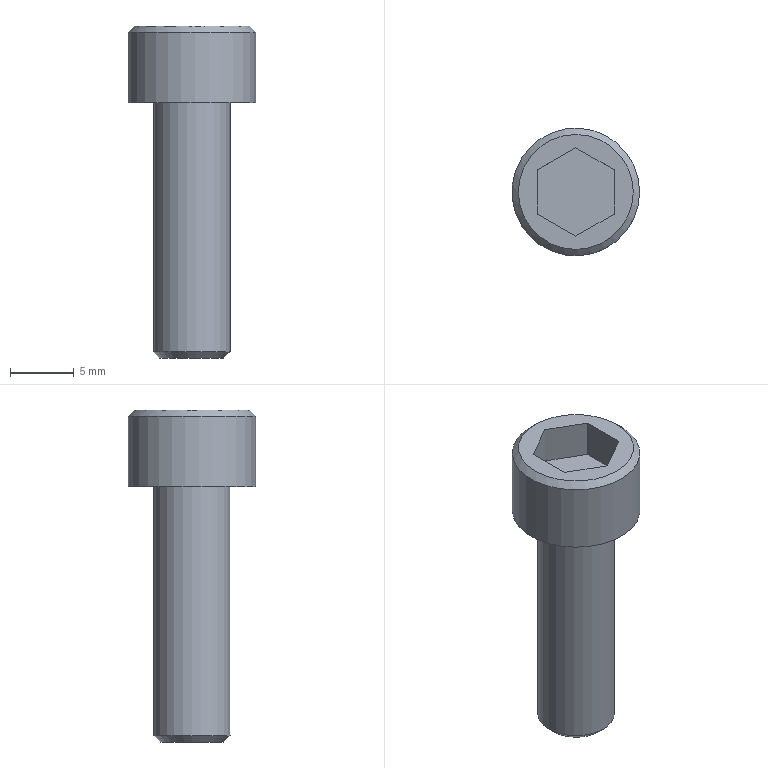Part | NX | features solid 2 | 1 solid | 14 faces | box 10 x 10 x 26 mm | volume 937.173 mm3 | plane 10 | cylinder 2 | cone 2 | commonest cylinder face diameters 6 x1 10 x1
STEP:
#1=CARTESIAN_POINT('',(47.,0.,109.5));
#2=VERTEX_POINT('',#1);
#3=CARTESIAN_POINT('',(42.5,0.,109.5));
#4=DIRECTION('',(0.,0.,1.));
#5=DIRECTION('',(1.,0.,0.));
#6=AXIS2_PLACEMENT_3D('',#3,#4,#5);
#7=CIRCLE('',#6,4.5);
#8=EDGE_CURVE('',#2,#2,#7,.T.);
#9=ORIENTED_EDGE('',*,*,#8,.T.);
#10=EDGE_LOOP('',(#9));
#11=FACE_BOUND('',#10,.T.);
#12=CARTESIAN_POINT('',(45.5,-1.732,109.5));
#13=VERTEX_POINT('',#12);
#14=CARTESIAN_POINT('',(42.5,-3.464,109.5));
#15=VERTEX_POINT('',#14);
#16=CARTESIAN_POINT('',(45.5,-1.732,109.5));
#17=DIRECTION('',(-0.866,-0.5,0.));
#18=VECTOR('',#17,1000.);
#19=LINE('',#16,#18);
#20=EDGE_CURVE('',#13,#15,#19,.T.);
#21=ORIENTED_EDGE('',*,*,#20,.T.);
#22=CARTESIAN_POINT('',(39.5,-1.732,109.5));
#23=VERTEX_POINT('',#22);
#24=CARTESIAN_POINT('',(42.5,-3.464,109.5));
#25=DIRECTION('',(-0.866,0.5,0.));
#26=VECTOR('',#25,1000.);
#27=LINE('',#24,#26);
#28=EDGE_CURVE('',#15,#23,#27,.T.);
#29=ORIENTED_EDGE('',*,*,#28,.T.);
#30=CARTESIAN_POINT('',(39.5,1.732,109.5));
#31=VERTEX_POINT('',#30);
#32=CARTESIAN_POINT('',(39.5,-1.732,109.5));
#33=DIRECTION('',(0.,1.,0.));
#34=VECTOR('',#33,1000.);
#35=LINE('',#32,#34);
#36=EDGE_CURVE('',#23,#31,#35,.T.);
#37=ORIENTED_EDGE('',*,*,#36,.T.);
#38=CARTESIAN_POINT('',(42.5,3.464,109.5));
#39=VERTEX_POINT('',#38);
#40=CARTESIAN_POINT('',(39.5,1.732,109.5));
#41=DIRECTION('',(0.866,0.5,0.));
#42=VECTOR('',#41,1000.);
#43=LINE('',#40,#42);
#44=EDGE_CURVE('',#31,#39,#43,.T.);
#45=ORIENTED_EDGE('',*,*,#44,.T.);
#46=CARTESIAN_POINT('',(45.5,1.732,109.5));
#47=VERTEX_POINT('',#46);
#48=CARTESIAN_POINT('',(42.5,3.464,109.5));
#49=DIRECTION('',(0.866,-0.5,0.));
#50=VECTOR('',#49,1000.);
#51=LINE('',#48,#50);
#52=EDGE_CURVE('',#39,#47,#51,.T.);
#53=ORIENTED_EDGE('',*,*,#52,.T.);
#54=CARTESIAN_POINT('',(45.5,1.732,109.5));
#55=DIRECTION('',(0.,-1.,0.));
#56=VECTOR('',#55,1000.);
#57=LINE('',#54,#56);
#58=EDGE_CURVE('',#47,#13,#57,.T.);
#59=ORIENTED_EDGE('',*,*,#58,.T.);
#60=EDGE_LOOP('',(#21,#29,#37,#45,#53,#59));
#61=FACE_BOUND('',#60,.T.);
#62=CARTESIAN_POINT('',(42.5,0.,109.5));
#63=DIRECTION('',(0.,0.,1.));
#64=DIRECTION('',(1.,0.,0.));
#65=AXIS2_PLACEMENT_3D('',#62,#63,#64);
#66=PLANE('',#65);
#67=ADVANCED_FACE('',(#11,#61),#66,.T.);
#68=CARTESIAN_POINT('',(40.,0.,83.5));
#69=VERTEX_POINT('',#68);
#70=CARTESIAN_POINT('',(42.5,0.,83.5));
#71=DIRECTION('',(0.,0.,-1.));
#72=DIRECTION('',(-1.,0.,0.));
#73=AXIS2_PLACEMENT_3D('',#70,#71,#72);
#74=CIRCLE('',#73,2.5);
#75=EDGE_CURVE('',#69,#69,#74,.T.);
#76=ORIENTED_EDGE('',*,*,#75,.T.);
#77=EDGE_LOOP('',(#76));
#78=FACE_BOUND('',#77,.T.);
#79=CARTESIAN_POINT('',(42.5,0.,83.5));
#80=DIRECTION('',(0.,0.,-1.));
#81=DIRECTION('',(-1.,0.,0.));
#82=AXIS2_PLACEMENT_3D('',#79,#80,#81);
#83=PLANE('',#82);
#84=ADVANCED_FACE('',(#78),#83,.T.);
#85=CARTESIAN_POINT('',(39.5,0.,84.));
#86=VERTEX_POINT('',#85);
#87=CARTESIAN_POINT('',(42.5,0.,84.));
#88=DIRECTION('',(0.,0.,-1.));
#89=DIRECTION('',(-1.,0.,0.));
#90=AXIS2_PLACEMENT_3D('',#87,#88,#89);
#91=CIRCLE('',#90,3.);
#92=EDGE_CURVE('',#86,#86,#91,.F.);
#93=ORIENTED_EDGE('',*,*,#92,.T.);
#94=EDGE_LOOP('',(#93));
#95=FACE_BOUND('',#94,.T.);
#96=CARTESIAN_POINT('',(45.5,0.,103.5));
#97=VERTEX_POINT('',#96);
#98=CARTESIAN_POINT('',(42.5,0.,103.5));
#99=DIRECTION('',(0.,0.,-1.));
#100=DIRECTION('',(1.,0.,0.));
#101=AXIS2_PLACEMENT_3D('',#98,#99,#100);
#102=CIRCLE('',#101,3.);
#103=EDGE_CURVE('',#97,#97,#102,.T.);
#104=ORIENTED_EDGE('',*,*,#103,.T.);
#105=EDGE_LOOP('',(#104));
#106=FACE_BOUND('',#105,.T.);
#107=CARTESIAN_POINT('',(42.5,0.,103.5));
#108=DIRECTION('',(0.,0.,-1.));
#109=DIRECTION('',(1.,0.,0.));
#110=AXIS2_PLACEMENT_3D('',#107,#108,#109);
#111=CYLINDRICAL_SURFACE('',#110,3.);
#112=ADVANCED_FACE('',(#95,#106),#111,.T.);
#113=CARTESIAN_POINT('',(47.5,0.,103.5));
#114=VERTEX_POINT('',#113);
#115=CARTESIAN_POINT('',(42.5,0.,103.5));
#116=DIRECTION('',(0.,0.,1.));
#117=DIRECTION('',(1.,0.,0.));
#118=AXIS2_PLACEMENT_3D('',#115,#116,#117);
#119=CIRCLE('',#118,5.);
#120=EDGE_CURVE('',#114,#114,#119,.T.);
#121=ORIENTED_EDGE('',*,*,#120,.F.);
#122=EDGE_LOOP('',(#121));
#123=FACE_BOUND('',#122,.T.);
#124=ORIENTED_EDGE('',*,*,#103,.F.);
#125=EDGE_LOOP('',(#124));
#126=FACE_BOUND('',#125,.T.);
#127=CARTESIAN_POINT('',(42.5,0.,103.5));
#128=DIRECTION('',(0.,0.,-1.));
#129=DIRECTION('',(-1.,0.,0.));
#130=AXIS2_PLACEMENT_3D('',#127,#128,#129);
#131=PLANE('',#130);
#132=ADVANCED_FACE('',(#123,#126),#131,.T.);
#133=CARTESIAN_POINT('',(47.5,0.,109.));
#134=VERTEX_POINT('',#133);
#135=CARTESIAN_POINT('',(42.5,0.,109.));
#136=DIRECTION('',(0.,0.,1.));
#137=DIRECTION('',(1.,0.,0.));
#138=AXIS2_PLACEMENT_3D('',#135,#136,#137);
#139=CIRCLE('',#138,5.);
#140=EDGE_CURVE('',#134,#134,#139,.F.);
#141=ORIENTED_EDGE('',*,*,#140,.T.);
#142=EDGE_LOOP('',(#141));
#143=FACE_BOUND('',#142,.T.);
#144=ORIENTED_EDGE('',*,*,#120,.T.);
#145=EDGE_LOOP('',(#144));
#146=FACE_BOUND('',#145,.T.);
#147=CARTESIAN_POINT('',(42.5,0.,103.5));
#148=DIRECTION('',(0.,0.,1.));
#149=DIRECTION('',(1.,0.,0.));
#150=AXIS2_PLACEMENT_3D('',#147,#148,#149);
#151=CYLINDRICAL_SURFACE('',#150,5.);
#152=ADVANCED_FACE('',(#143,#146),#151,.T.);
#153=CARTESIAN_POINT('',(42.5,-3.464,106.5));
#154=VERTEX_POINT('',#153);
#155=CARTESIAN_POINT('',(45.5,-1.732,106.5));
#156=VERTEX_POINT('',#155);
#157=CARTESIAN_POINT('',(45.5,-1.732,106.5));
#158=DIRECTION('',(-0.866,-0.5,0.));
#159=VECTOR('',#158,1000.);
#160=LINE('',#157,#159);
#161=EDGE_CURVE('',#154,#156,#160,.F.);
#162=ORIENTED_EDGE('',*,*,#161,.F.);
#163=CARTESIAN_POINT('',(42.5,-3.464,109.5));
#164=DIRECTION('',(0.,0.,-1.));
#165=VECTOR('',#164,1000.);
#166=LINE('',#163,#165);
#167=EDGE_CURVE('',#154,#15,#166,.F.);
#168=ORIENTED_EDGE('',*,*,#167,.T.);
#169=ORIENTED_EDGE('',*,*,#20,.F.);
#170=CARTESIAN_POINT('',(45.5,-1.732,109.5));
#171=DIRECTION('',(0.,0.,-1.));
#172=VECTOR('',#171,1000.);
#173=LINE('',#170,#172);
#174=EDGE_CURVE('',#156,#13,#173,.F.);
#175=ORIENTED_EDGE('',*,*,#174,.F.);
#176=EDGE_LOOP('',(#162,#168,#169,#175));
#177=FACE_BOUND('',#176,.T.);
#178=CARTESIAN_POINT('',(44.,-2.598,108.));
#179=DIRECTION('',(0.5,-0.866,0.));
#180=DIRECTION('',(0.866,0.5,0.));
#181=AXIS2_PLACEMENT_3D('',#178,#179,#180);
#182=PLANE('',#181);
#183=ADVANCED_FACE('',(#177),#182,.F.);
#184=CARTESIAN_POINT('',(45.5,1.732,106.5));
#185=VERTEX_POINT('',#184);
#186=CARTESIAN_POINT('',(45.5,1.732,106.5));
#187=DIRECTION('',(0.,-1.,0.));
#188=VECTOR('',#187,1000.);
#189=LINE('',#186,#188);
#190=EDGE_CURVE('',#156,#185,#189,.F.);
#191=ORIENTED_EDGE('',*,*,#190,.F.);
#192=ORIENTED_EDGE('',*,*,#174,.T.);
#193=ORIENTED_EDGE('',*,*,#58,.F.);
#194=CARTESIAN_POINT('',(45.5,1.732,109.5));
#195=DIRECTION('',(0.,0.,-1.));
#196=VECTOR('',#195,1000.);
#197=LINE('',#194,#196);
#198=EDGE_CURVE('',#185,#47,#197,.F.);
#199=ORIENTED_EDGE('',*,*,#198,.F.);
#200=EDGE_LOOP('',(#191,#192,#193,#199));
#201=FACE_BOUND('',#200,.T.);
#202=CARTESIAN_POINT('',(45.5,0.,108.));
#203=DIRECTION('',(1.,0.,0.));
#204=DIRECTION('',(0.,0.,-1.));
#205=AXIS2_PLACEMENT_3D('',#202,#203,#204);
#206=PLANE('',#205);
#207=ADVANCED_FACE('',(#201),#206,.F.);
#208=CARTESIAN_POINT('',(42.5,3.464,106.5));
#209=VERTEX_POINT('',#208);
#210=CARTESIAN_POINT('',(42.5,3.464,106.5));
#211=DIRECTION('',(0.866,-0.5,0.));
#212=VECTOR('',#211,1000.);
#213=LINE('',#210,#212);
#214=EDGE_CURVE('',#185,#209,#213,.F.);
#215=ORIENTED_EDGE('',*,*,#214,.F.);
#216=ORIENTED_EDGE('',*,*,#198,.T.);
#217=ORIENTED_EDGE('',*,*,#52,.F.);
#218=CARTESIAN_POINT('',(42.5,3.464,109.5));
#219=DIRECTION('',(0.,0.,-1.));
#220=VECTOR('',#219,1000.);
#221=LINE('',#218,#220);
#222=EDGE_CURVE('',#209,#39,#221,.F.);
#223=ORIENTED_EDGE('',*,*,#222,.F.);
#224=EDGE_LOOP('',(#215,#216,#217,#223));
#225=FACE_BOUND('',#224,.T.);
#226=CARTESIAN_POINT('',(44.,2.598,108.));
#227=DIRECTION('',(0.5,0.866,0.));
#228=DIRECTION('',(-0.866,0.5,0.));
#229=AXIS2_PLACEMENT_3D('',#226,#227,#228);
#230=PLANE('',#229);
#231=ADVANCED_FACE('',(#225),#230,.F.);
#232=CARTESIAN_POINT('',(39.5,1.732,106.5));
#233=VERTEX_POINT('',#232);
#234=CARTESIAN_POINT('',(39.5,1.732,106.5));
#235=DIRECTION('',(0.866,0.5,0.));
#236=VECTOR('',#235,1000.);
#237=LINE('',#234,#236);
#238=EDGE_CURVE('',#209,#233,#237,.F.);
#239=ORIENTED_EDGE('',*,*,#238,.F.);
#240=ORIENTED_EDGE('',*,*,#222,.T.);
#241=ORIENTED_EDGE('',*,*,#44,.F.);
#242=CARTESIAN_POINT('',(39.5,1.732,109.5));
#243=DIRECTION('',(0.,0.,-1.));
#244=VECTOR('',#243,1000.);
#245=LINE('',#242,#244);
#246=EDGE_CURVE('',#233,#31,#245,.F.);
#247=ORIENTED_EDGE('',*,*,#246,.F.);
#248=EDGE_LOOP('',(#239,#240,#241,#247));
#249=FACE_BOUND('',#248,.T.);
#250=CARTESIAN_POINT('',(41.,2.598,108.));
#251=DIRECTION('',(-0.5,0.866,0.));
#252=DIRECTION('',(-0.866,-0.5,0.));
#253=AXIS2_PLACEMENT_3D('',#250,#251,#252);
#254=PLANE('',#253);
#255=ADVANCED_FACE('',(#249),#254,.F.);
#256=CARTESIAN_POINT('',(39.5,-1.732,106.5));
#257=VERTEX_POINT('',#256);
#258=CARTESIAN_POINT('',(39.5,-1.732,106.5));
#259=DIRECTION('',(0.,1.,0.));
#260=VECTOR('',#259,1000.);
#261=LINE('',#258,#260);
#262=EDGE_CURVE('',#233,#257,#261,.F.);
#263=ORIENTED_EDGE('',*,*,#262,.F.);
#264=ORIENTED_EDGE('',*,*,#246,.T.);
#265=ORIENTED_EDGE('',*,*,#36,.F.);
#266=CARTESIAN_POINT('',(39.5,-1.732,109.5));
#267=DIRECTION('',(0.,0.,-1.));
#268=VECTOR('',#267,1000.);
#269=LINE('',#266,#268);
#270=EDGE_CURVE('',#257,#23,#269,.F.);
#271=ORIENTED_EDGE('',*,*,#270,.F.);
#272=EDGE_LOOP('',(#263,#264,#265,#271));
#273=FACE_BOUND('',#272,.T.);
#274=CARTESIAN_POINT('',(39.5,0.,108.));
#275=DIRECTION('',(-1.,0.,0.));
#276=DIRECTION('',(0.,0.,1.));
#277=AXIS2_PLACEMENT_3D('',#274,#275,#276);
#278=PLANE('',#277);
#279=ADVANCED_FACE('',(#273),#278,.F.);
#280=CARTESIAN_POINT('',(42.5,-3.464,106.5));
#281=DIRECTION('',(-0.866,0.5,0.));
#282=VECTOR('',#281,1000.);
#283=LINE('',#280,#282);
#284=EDGE_CURVE('',#257,#154,#283,.F.);
#285=ORIENTED_EDGE('',*,*,#284,.F.);
#286=ORIENTED_EDGE('',*,*,#270,.T.);
#287=ORIENTED_EDGE('',*,*,#28,.F.);
#288=ORIENTED_EDGE('',*,*,#167,.F.);
#289=EDGE_LOOP('',(#285,#286,#287,#288));
#290=FACE_BOUND('',#289,.T.);
#291=CARTESIAN_POINT('',(41.,-2.598,108.));
#292=DIRECTION('',(-0.5,-0.866,0.));
#293=DIRECTION('',(0.866,-0.5,0.));
#294=AXIS2_PLACEMENT_3D('',#291,#292,#293);
#295=PLANE('',#294);
#296=ADVANCED_FACE('',(#290),#295,.F.);
#297=ORIENTED_EDGE('',*,*,#190,.T.);
#298=ORIENTED_EDGE('',*,*,#214,.T.);
#299=ORIENTED_EDGE('',*,*,#238,.T.);
#300=ORIENTED_EDGE('',*,*,#262,.T.);
#301=ORIENTED_EDGE('',*,*,#284,.T.);
#302=ORIENTED_EDGE('',*,*,#161,.T.);
#303=EDGE_LOOP('',(#297,#298,#299,#300,#301,#302));
#304=FACE_BOUND('',#303,.T.);
#305=CARTESIAN_POINT('',(42.5,0.,106.5));
#306=DIRECTION('',(0.,0.,-1.));
#307=DIRECTION('',(-1.,0.,0.));
#308=AXIS2_PLACEMENT_3D('',#305,#306,#307);
#309=PLANE('',#308);
#310=ADVANCED_FACE('',(#304),#309,.F.);
#311=ORIENTED_EDGE('',*,*,#75,.F.);
#312=EDGE_LOOP('',(#311));
#313=FACE_BOUND('',#312,.T.);
#314=ORIENTED_EDGE('',*,*,#92,.F.);
#315=EDGE_LOOP('',(#314));
#316=FACE_BOUND('',#315,.T.);
#317=CARTESIAN_POINT('',(42.5,0.,84.));
#318=DIRECTION('',(0.,0.,1.));
#319=DIRECTION('',(1.,0.,0.));
#320=AXIS2_PLACEMENT_3D('',#317,#318,#319);
#321=CONICAL_SURFACE('',#320,3.,0.7854);
#322=ADVANCED_FACE('',(#313,#316),#321,.T.);
#323=ORIENTED_EDGE('',*,*,#8,.F.);
#324=EDGE_LOOP('',(#323));
#325=FACE_BOUND('',#324,.T.);
#326=ORIENTED_EDGE('',*,*,#140,.F.);
#327=EDGE_LOOP('',(#326));
#328=FACE_BOUND('',#327,.T.);
#329=CARTESIAN_POINT('',(42.5,0.,109.));
#330=DIRECTION('',(0.,0.,-1.));
#331=DIRECTION('',(-1.,0.,0.));
#332=AXIS2_PLACEMENT_3D('',#329,#330,#331);
#333=CONICAL_SURFACE('',#332,5.,0.7854);
#334=ADVANCED_FACE('',(#325,#328),#333,.T.);
#335=CLOSED_SHELL('',(#67,#84,#112,#132,#152,#183,#207,#231,#255,#279,#296,#310,#322,#334));
#336=MANIFOLD_SOLID_BREP('',#335);
#337=(LENGTH_UNIT()NAMED_UNIT(*)SI_UNIT(.MILLI.,.METRE.));
#338=UNCERTAINTY_MEASURE_WITH_UNIT(LENGTH_MEASURE(0.00001),#337,'','');
#339=(NAMED_UNIT(*)PLANE_ANGLE_UNIT()SI_UNIT($,.RADIAN.));
#340=(NAMED_UNIT(*)SI_UNIT($,.STERADIAN.)SOLID_ANGLE_UNIT());
#341=(GEOMETRIC_REPRESENTATION_CONTEXT(3)GLOBAL_UNCERTAINTY_ASSIGNED_CONTEXT((#338))GLOBAL_UNIT_ASSIGNED_CONTEXT((#337,#339,#340))REPRESENTATION_CONTEXT('',''));
#342=ADVANCED_BREP_SHAPE_REPRESENTATION('',(#336),#341);